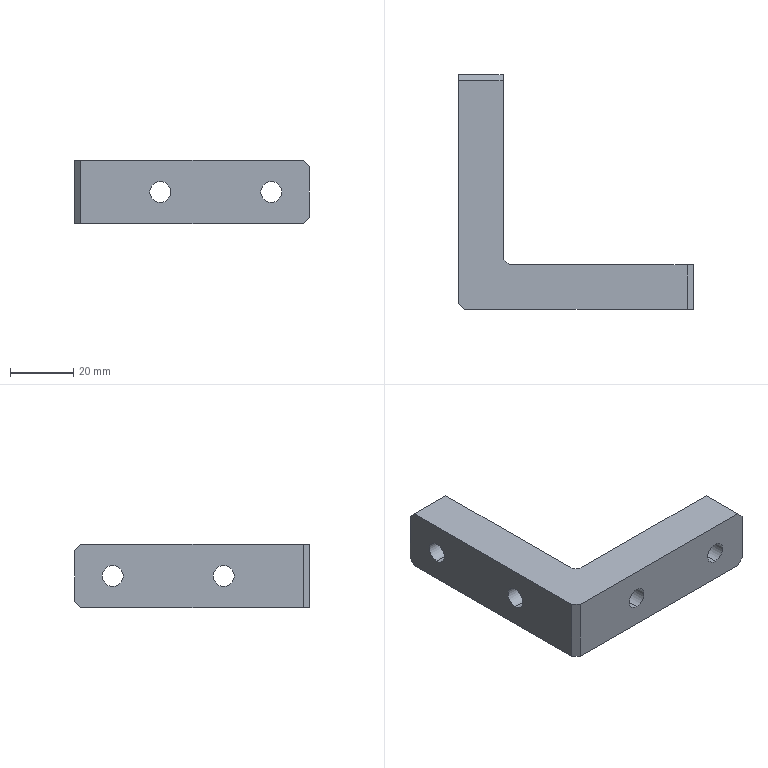Part | SolidWorks | features 3DProfileFeature 2, Chamfer 2, HoleWzd 2, Extrusion 1, Fillet 1 | 1 solid | 42 faces | box 74 x 74 x 20 mm | volume 33836 mm3 | cylinder 17 | plane 17 | cone 8 | commonest cylinder face diameters 6.6 x8 11 x8 6 x1
STEP:
#1=CARTESIAN_POINT('',(-12.,13.975,-5.5));
#2=VERTEX_POINT('',#1);
#3=CARTESIAN_POINT('',(-12.,13.975,5.5));
#4=VERTEX_POINT('',#3);
#5=CARTESIAN_POINT('',(-12.,13.975,0.));
#6=DIRECTION('',(0.,1.,0.));
#7=DIRECTION('',(0.,0.,1.));
#8=AXIS2_PLACEMENT_3D('',#5,#6,#7);
#9=CIRCLE('',#8,5.5);
#10=EDGE_CURVE('',#2,#4,#9,.T.);
#11=ORIENTED_EDGE('',*,*,#10,.F.);
#12=CARTESIAN_POINT('',(-12.,14.,-5.525));
#13=VERTEX_POINT('',#12);
#14=CARTESIAN_POINT('',(-12.,14.,-5.525));
#15=DIRECTION('',(0.,0.7071,-0.7071));
#16=VECTOR('',#15,1000.);
#17=LINE('',#14,#16);
#18=EDGE_CURVE('',#2,#13,#17,.T.);
#19=ORIENTED_EDGE('',*,*,#18,.T.);
#20=CARTESIAN_POINT('',(-12.,14.,5.525));
#21=VERTEX_POINT('',#20);
#22=CARTESIAN_POINT('',(-12.,14.,0.));
#23=DIRECTION('',(0.,1.,0.));
#24=DIRECTION('',(0.,0.,1.));
#25=AXIS2_PLACEMENT_3D('',#22,#23,#24);
#26=CIRCLE('',#25,5.525);
#27=EDGE_CURVE('',#13,#21,#26,.T.);
#28=ORIENTED_EDGE('',*,*,#27,.T.);
#29=CARTESIAN_POINT('',(-12.,14.,5.525));
#30=DIRECTION('',(0.,0.7071,0.7071));
#31=VECTOR('',#30,1000.);
#32=LINE('',#29,#31);
#33=EDGE_CURVE('',#4,#21,#32,.T.);
#34=ORIENTED_EDGE('',*,*,#33,.F.);
#35=EDGE_LOOP('',(#11,#19,#28,#34));
#36=FACE_OUTER_BOUND('',#35,.T.);
#37=CARTESIAN_POINT('',(-12.,14.,0.));
#38=DIRECTION('',(0.,1.,0.));
#39=DIRECTION('',(0.,0.,1.));
#40=AXIS2_PLACEMENT_3D('',#37,#38,#39);
#41=CONICAL_SURFACE('',#40,5.525,0.7854);
#42=ADVANCED_FACE('',(#36),#41,.F.);
#43=CARTESIAN_POINT('',(-12.,7.2,-5.5));
#44=VERTEX_POINT('',#43);
#45=CARTESIAN_POINT('',(-12.,7.2,5.5));
#46=VERTEX_POINT('',#45);
#47=CARTESIAN_POINT('',(-12.,7.2,0.));
#48=DIRECTION('',(0.,1.,0.));
#49=DIRECTION('',(0.,0.,1.));
#50=AXIS2_PLACEMENT_3D('',#47,#48,#49);
#51=CIRCLE('',#50,5.5);
#52=EDGE_CURVE('',#44,#46,#51,.T.);
#53=ORIENTED_EDGE('',*,*,#52,.F.);
#54=CARTESIAN_POINT('',(-12.,14.,-5.5));
#55=DIRECTION('',(0.,1.,0.));
#56=VECTOR('',#55,1000.);
#57=LINE('',#54,#56);
#58=EDGE_CURVE('',#44,#2,#57,.T.);
#59=ORIENTED_EDGE('',*,*,#58,.T.);
#60=ORIENTED_EDGE('',*,*,#10,.T.);
#61=CARTESIAN_POINT('',(-12.,14.,5.5));
#62=DIRECTION('',(0.,1.,0.));
#63=VECTOR('',#62,1000.);
#64=LINE('',#61,#63);
#65=EDGE_CURVE('',#46,#4,#64,.T.);
#66=ORIENTED_EDGE('',*,*,#65,.F.);
#67=EDGE_LOOP('',(#53,#59,#60,#66));
#68=FACE_OUTER_BOUND('',#67,.T.);
#69=CARTESIAN_POINT('',(-12.,14.,0.));
#70=DIRECTION('',(0.,1.,0.));
#71=DIRECTION('',(0.,0.,1.));
#72=AXIS2_PLACEMENT_3D('',#69,#70,#71);
#73=CYLINDRICAL_SURFACE('',#72,5.5);
#74=ADVANCED_FACE('',(#68),#73,.F.);
#75=CARTESIAN_POINT('',(-12.,0.,-3.3));
#76=VERTEX_POINT('',#75);
#77=CARTESIAN_POINT('',(-12.,0.,3.3));
#78=VERTEX_POINT('',#77);
#79=CARTESIAN_POINT('',(-12.,0.,0.));
#80=DIRECTION('',(0.,1.,0.));
#81=DIRECTION('',(-1.,0.,0.));
#82=AXIS2_PLACEMENT_3D('',#79,#80,#81);
#83=CIRCLE('',#82,3.3);
#84=EDGE_CURVE('',#76,#78,#83,.T.);
#85=ORIENTED_EDGE('',*,*,#84,.F.);
#86=CARTESIAN_POINT('',(-12.,7.2,-3.3));
#87=VERTEX_POINT('',#86);
#88=CARTESIAN_POINT('',(-12.,14.,-3.3));
#89=DIRECTION('',(0.,1.,0.));
#90=VECTOR('',#89,1000.);
#91=LINE('',#88,#90);
#92=EDGE_CURVE('',#76,#87,#91,.T.);
#93=ORIENTED_EDGE('',*,*,#92,.T.);
#94=CARTESIAN_POINT('',(-12.,7.2,3.3));
#95=VERTEX_POINT('',#94);
#96=CARTESIAN_POINT('',(-12.,7.2,0.));
#97=DIRECTION('',(0.,1.,0.));
#98=DIRECTION('',(0.,0.,1.));
#99=AXIS2_PLACEMENT_3D('',#96,#97,#98);
#100=CIRCLE('',#99,3.3);
#101=EDGE_CURVE('',#87,#95,#100,.T.);
#102=ORIENTED_EDGE('',*,*,#101,.T.);
#103=CARTESIAN_POINT('',(-12.,14.,3.3));
#104=DIRECTION('',(0.,1.,0.));
#105=VECTOR('',#104,1000.);
#106=LINE('',#103,#105);
#107=EDGE_CURVE('',#78,#95,#106,.T.);
#108=ORIENTED_EDGE('',*,*,#107,.F.);
#109=EDGE_LOOP('',(#85,#93,#102,#108));
#110=FACE_OUTER_BOUND('',#109,.T.);
#111=CARTESIAN_POINT('',(-12.,14.,0.));
#112=DIRECTION('',(0.,1.,0.));
#113=DIRECTION('',(0.,0.,1.));
#114=AXIS2_PLACEMENT_3D('',#111,#112,#113);
#115=CYLINDRICAL_SURFACE('',#114,3.3);
#116=ADVANCED_FACE('',(#110),#115,.F.);
#117=CARTESIAN_POINT('',(-47.,13.975,-5.5));
#118=VERTEX_POINT('',#117);
#119=CARTESIAN_POINT('',(-47.,13.975,5.5));
#120=VERTEX_POINT('',#119);
#121=CARTESIAN_POINT('',(-47.,13.975,0.));
#122=DIRECTION('',(0.,1.,0.));
#123=DIRECTION('',(0.,0.,1.));
#124=AXIS2_PLACEMENT_3D('',#121,#122,#123);
#125=CIRCLE('',#124,5.5);
#126=EDGE_CURVE('',#118,#120,#125,.T.);
#127=ORIENTED_EDGE('',*,*,#126,.F.);
#128=CARTESIAN_POINT('',(-47.,14.,-5.525));
#129=VERTEX_POINT('',#128);
#130=CARTESIAN_POINT('',(-47.,14.,-5.525));
#131=DIRECTION('',(0.,0.7071,-0.7071));
#132=VECTOR('',#131,1000.);
#133=LINE('',#130,#132);
#134=EDGE_CURVE('',#118,#129,#133,.T.);
#135=ORIENTED_EDGE('',*,*,#134,.T.);
#136=CARTESIAN_POINT('',(-47.,14.,5.525));
#137=VERTEX_POINT('',#136);
#138=CARTESIAN_POINT('',(-47.,14.,0.));
#139=DIRECTION('',(0.,1.,0.));
#140=DIRECTION('',(0.,0.,1.));
#141=AXIS2_PLACEMENT_3D('',#138,#139,#140);
#142=CIRCLE('',#141,5.525);
#143=EDGE_CURVE('',#129,#137,#142,.T.);
#144=ORIENTED_EDGE('',*,*,#143,.T.);
#145=CARTESIAN_POINT('',(-47.,14.,5.525));
#146=DIRECTION('',(0.,0.7071,0.7071));
#147=VECTOR('',#146,1000.);
#148=LINE('',#145,#147);
#149=EDGE_CURVE('',#120,#137,#148,.T.);
#150=ORIENTED_EDGE('',*,*,#149,.F.);
#151=EDGE_LOOP('',(#127,#135,#144,#150));
#152=FACE_OUTER_BOUND('',#151,.T.);
#153=CARTESIAN_POINT('',(-47.,14.,0.));
#154=DIRECTION('',(0.,1.,0.));
#155=DIRECTION('',(0.,0.,1.));
#156=AXIS2_PLACEMENT_3D('',#153,#154,#155);
#157=CONICAL_SURFACE('',#156,5.525,0.7854);
#158=ADVANCED_FACE('',(#152),#157,.F.);
#159=CARTESIAN_POINT('',(-47.,7.2,-5.5));
#160=VERTEX_POINT('',#159);
#161=CARTESIAN_POINT('',(-47.,7.2,5.5));
#162=VERTEX_POINT('',#161);
#163=CARTESIAN_POINT('',(-47.,7.2,0.));
#164=DIRECTION('',(0.,1.,0.));
#165=DIRECTION('',(0.,0.,1.));
#166=AXIS2_PLACEMENT_3D('',#163,#164,#165);
#167=CIRCLE('',#166,5.5);
#168=EDGE_CURVE('',#160,#162,#167,.T.);
#169=ORIENTED_EDGE('',*,*,#168,.F.);
#170=CARTESIAN_POINT('',(-47.,14.,-5.5));
#171=DIRECTION('',(0.,1.,0.));
#172=VECTOR('',#171,1000.);
#173=LINE('',#170,#172);
#174=EDGE_CURVE('',#160,#118,#173,.T.);
#175=ORIENTED_EDGE('',*,*,#174,.T.);
#176=ORIENTED_EDGE('',*,*,#126,.T.);
#177=CARTESIAN_POINT('',(-47.,14.,5.5));
#178=DIRECTION('',(0.,1.,0.));
#179=VECTOR('',#178,1000.);
#180=LINE('',#177,#179);
#181=EDGE_CURVE('',#162,#120,#180,.T.);
#182=ORIENTED_EDGE('',*,*,#181,.F.);
#183=EDGE_LOOP('',(#169,#175,#176,#182));
#184=FACE_OUTER_BOUND('',#183,.T.);
#185=CARTESIAN_POINT('',(-47.,14.,0.));
#186=DIRECTION('',(0.,1.,0.));
#187=DIRECTION('',(0.,0.,1.));
#188=AXIS2_PLACEMENT_3D('',#185,#186,#187);
#189=CYLINDRICAL_SURFACE('',#188,5.5);
#190=ADVANCED_FACE('',(#184),#189,.F.);
#191=CARTESIAN_POINT('',(-47.,0.,-3.3));
#192=VERTEX_POINT('',#191);
#193=CARTESIAN_POINT('',(-47.,0.,3.3));
#194=VERTEX_POINT('',#193);
#195=CARTESIAN_POINT('',(-47.,0.,0.));
#196=DIRECTION('',(0.,1.,0.));
#197=DIRECTION('',(-1.,0.,0.));
#198=AXIS2_PLACEMENT_3D('',#195,#196,#197);
#199=CIRCLE('',#198,3.3);
#200=EDGE_CURVE('',#192,#194,#199,.T.);
#201=ORIENTED_EDGE('',*,*,#200,.F.);
#202=CARTESIAN_POINT('',(-47.,7.2,-3.3));
#203=VERTEX_POINT('',#202);
#204=CARTESIAN_POINT('',(-47.,14.,-3.3));
#205=DIRECTION('',(0.,1.,0.));
#206=VECTOR('',#205,1000.);
#207=LINE('',#204,#206);
#208=EDGE_CURVE('',#192,#203,#207,.T.);
#209=ORIENTED_EDGE('',*,*,#208,.T.);
#210=CARTESIAN_POINT('',(-47.,7.2,3.3));
#211=VERTEX_POINT('',#210);
#212=CARTESIAN_POINT('',(-47.,7.2,0.));
#213=DIRECTION('',(0.,1.,0.));
#214=DIRECTION('',(0.,0.,1.));
#215=AXIS2_PLACEMENT_3D('',#212,#213,#214);
#216=CIRCLE('',#215,3.3);
#217=EDGE_CURVE('',#203,#211,#216,.T.);
#218=ORIENTED_EDGE('',*,*,#217,.T.);
#219=CARTESIAN_POINT('',(-47.,14.,3.3));
#220=DIRECTION('',(0.,1.,0.));
#221=VECTOR('',#220,1000.);
#222=LINE('',#219,#221);
#223=EDGE_CURVE('',#194,#211,#222,.T.);
#224=ORIENTED_EDGE('',*,*,#223,.F.);
#225=EDGE_LOOP('',(#201,#209,#218,#224));
#226=FACE_OUTER_BOUND('',#225,.T.);
#227=CARTESIAN_POINT('',(-47.,14.,0.));
#228=DIRECTION('',(0.,1.,0.));
#229=DIRECTION('',(0.,0.,1.));
#230=AXIS2_PLACEMENT_3D('',#227,#228,#229);
#231=CYLINDRICAL_SURFACE('',#230,3.3);
#232=ADVANCED_FACE('',(#226),#231,.F.);
#233=CARTESIAN_POINT('',(-60.025,62.,5.5));
#234=VERTEX_POINT('',#233);
#235=CARTESIAN_POINT('',(-60.025,62.,-5.5));
#236=VERTEX_POINT('',#235);
#237=CARTESIAN_POINT('',(-60.025,62.,0.));
#238=DIRECTION('',(1.,0.,0.));
#239=DIRECTION('',(0.,0.,-1.));
#240=AXIS2_PLACEMENT_3D('',#237,#238,#239);
#241=CIRCLE('',#240,5.5);
#242=EDGE_CURVE('',#234,#236,#241,.T.);
#243=ORIENTED_EDGE('',*,*,#242,.F.);
#244=CARTESIAN_POINT('',(-60.,62.,5.525));
#245=VERTEX_POINT('',#244);
#246=CARTESIAN_POINT('',(-60.,62.,5.525));
#247=DIRECTION('',(0.7071,0.,0.7071));
#248=VECTOR('',#247,1000.);
#249=LINE('',#246,#248);
#250=EDGE_CURVE('',#234,#245,#249,.T.);
#251=ORIENTED_EDGE('',*,*,#250,.T.);
#252=CARTESIAN_POINT('',(-60.,62.,-5.525));
#253=VERTEX_POINT('',#252);
#254=CARTESIAN_POINT('',(-60.,62.,0.));
#255=DIRECTION('',(1.,0.,0.));
#256=DIRECTION('',(0.,0.,-1.));
#257=AXIS2_PLACEMENT_3D('',#254,#255,#256);
#258=CIRCLE('',#257,5.525);
#259=EDGE_CURVE('',#245,#253,#258,.T.);
#260=ORIENTED_EDGE('',*,*,#259,.T.);
#261=CARTESIAN_POINT('',(-60.,62.,-5.525));
#262=DIRECTION('',(0.7071,0.,-0.7071));
#263=VECTOR('',#262,1000.);
#264=LINE('',#261,#263);
#265=EDGE_CURVE('',#236,#253,#264,.T.);
#266=ORIENTED_EDGE('',*,*,#265,.F.);
#267=EDGE_LOOP('',(#243,#251,#260,#266));
#268=FACE_OUTER_BOUND('',#267,.T.);
#269=CARTESIAN_POINT('',(-60.,62.,0.));
#270=DIRECTION('',(1.,0.,0.));
#271=DIRECTION('',(0.,0.,-1.));
#272=AXIS2_PLACEMENT_3D('',#269,#270,#271);
#273=CONICAL_SURFACE('',#272,5.525,0.7854);
#274=ADVANCED_FACE('',(#268),#273,.F.);
#275=CARTESIAN_POINT('',(-66.8,62.,5.5));
#276=VERTEX_POINT('',#275);
#277=CARTESIAN_POINT('',(-66.8,62.,-5.5));
#278=VERTEX_POINT('',#277);
#279=CARTESIAN_POINT('',(-66.8,62.,0.));
#280=DIRECTION('',(1.,0.,0.));
#281=DIRECTION('',(0.,0.,-1.));
#282=AXIS2_PLACEMENT_3D('',#279,#280,#281);
#283=CIRCLE('',#282,5.5);
#284=EDGE_CURVE('',#276,#278,#283,.T.);
#285=ORIENTED_EDGE('',*,*,#284,.F.);
#286=CARTESIAN_POINT('',(-60.,62.,5.5));
#287=DIRECTION('',(1.,0.,0.));
#288=VECTOR('',#287,1000.);
#289=LINE('',#286,#288);
#290=EDGE_CURVE('',#276,#234,#289,.T.);
#291=ORIENTED_EDGE('',*,*,#290,.T.);
#292=ORIENTED_EDGE('',*,*,#242,.T.);
#293=CARTESIAN_POINT('',(-60.,62.,-5.5));
#294=DIRECTION('',(1.,0.,0.));
#295=VECTOR('',#294,1000.);
#296=LINE('',#293,#295);
#297=EDGE_CURVE('',#278,#236,#296,.T.);
#298=ORIENTED_EDGE('',*,*,#297,.F.);
#299=EDGE_LOOP('',(#285,#291,#292,#298));
#300=FACE_OUTER_BOUND('',#299,.T.);
#301=CARTESIAN_POINT('',(-60.,62.,0.));
#302=DIRECTION('',(1.,0.,0.));
#303=DIRECTION('',(0.,0.,-1.));
#304=AXIS2_PLACEMENT_3D('',#301,#302,#303);
#305=CYLINDRICAL_SURFACE('',#304,5.5);
#306=ADVANCED_FACE('',(#300),#305,.F.);
#307=CARTESIAN_POINT('',(-74.,62.,3.3));
#308=VERTEX_POINT('',#307);
#309=CARTESIAN_POINT('',(-74.,62.,-3.3));
#310=VERTEX_POINT('',#309);
#311=CARTESIAN_POINT('',(-74.,62.,0.));
#312=DIRECTION('',(1.,0.,0.));
#313=DIRECTION('',(0.,0.,-1.));
#314=AXIS2_PLACEMENT_3D('',#311,#312,#313);
#315=CIRCLE('',#314,3.3);
#316=EDGE_CURVE('',#308,#310,#315,.T.);
#317=ORIENTED_EDGE('',*,*,#316,.F.);
#318=CARTESIAN_POINT('',(-66.8,62.,3.3));
#319=VERTEX_POINT('',#318);
#320=CARTESIAN_POINT('',(-60.,62.,3.3));
#321=DIRECTION('',(1.,0.,0.));
#322=VECTOR('',#321,1000.);
#323=LINE('',#320,#322);
#324=EDGE_CURVE('',#308,#319,#323,.T.);
#325=ORIENTED_EDGE('',*,*,#324,.T.);
#326=CARTESIAN_POINT('',(-66.8,62.,-3.3));
#327=VERTEX_POINT('',#326);
#328=CARTESIAN_POINT('',(-66.8,62.,0.));
#329=DIRECTION('',(1.,0.,0.));
#330=DIRECTION('',(0.,0.,-1.));
#331=AXIS2_PLACEMENT_3D('',#328,#329,#330);
#332=CIRCLE('',#331,3.3);
#333=EDGE_CURVE('',#319,#327,#332,.T.);
#334=ORIENTED_EDGE('',*,*,#333,.T.);
#335=CARTESIAN_POINT('',(-60.,62.,-3.3));
#336=DIRECTION('',(1.,0.,0.));
#337=VECTOR('',#336,1000.);
#338=LINE('',#335,#337);
#339=EDGE_CURVE('',#310,#327,#338,.T.);
#340=ORIENTED_EDGE('',*,*,#339,.F.);
#341=EDGE_LOOP('',(#317,#325,#334,#340));
#342=FACE_OUTER_BOUND('',#341,.T.);
#343=CARTESIAN_POINT('',(-60.,62.,0.));
#344=DIRECTION('',(1.,0.,0.));
#345=DIRECTION('',(0.,0.,-1.));
#346=AXIS2_PLACEMENT_3D('',#343,#344,#345);
#347=CYLINDRICAL_SURFACE('',#346,3.3);
#348=ADVANCED_FACE('',(#342),#347,.F.);
#349=CARTESIAN_POINT('',(-60.025,27.,5.5));
#350=VERTEX_POINT('',#349);
#351=CARTESIAN_POINT('',(-60.025,27.,-5.5));
#352=VERTEX_POINT('',#351);
#353=CARTESIAN_POINT('',(-60.025,27.,0.));
#354=DIRECTION('',(1.,0.,0.));
#355=DIRECTION('',(0.,0.,-1.));
#356=AXIS2_PLACEMENT_3D('',#353,#354,#355);
#357=CIRCLE('',#356,5.5);
#358=EDGE_CURVE('',#350,#352,#357,.T.);
#359=ORIENTED_EDGE('',*,*,#358,.F.);
#360=CARTESIAN_POINT('',(-60.,27.,5.525));
#361=VERTEX_POINT('',#360);
#362=CARTESIAN_POINT('',(-60.,27.,5.525));
#363=DIRECTION('',(0.7071,0.,0.7071));
#364=VECTOR('',#363,1000.);
#365=LINE('',#362,#364);
#366=EDGE_CURVE('',#350,#361,#365,.T.);
#367=ORIENTED_EDGE('',*,*,#366,.T.);
#368=CARTESIAN_POINT('',(-60.,27.,-5.525));
#369=VERTEX_POINT('',#368);
#370=CARTESIAN_POINT('',(-60.,27.,0.));
#371=DIRECTION('',(1.,0.,0.));
#372=DIRECTION('',(0.,0.,-1.));
#373=AXIS2_PLACEMENT_3D('',#370,#371,#372);
#374=CIRCLE('',#373,5.525);
#375=EDGE_CURVE('',#361,#369,#374,.T.);
#376=ORIENTED_EDGE('',*,*,#375,.T.);
#377=CARTESIAN_POINT('',(-60.,27.,-5.525));
#378=DIRECTION('',(0.7071,0.,-0.7071));
#379=VECTOR('',#378,1000.);
#380=LINE('',#377,#379);
#381=EDGE_CURVE('',#352,#369,#380,.T.);
#382=ORIENTED_EDGE('',*,*,#381,.F.);
#383=EDGE_LOOP('',(#359,#367,#376,#382));
#384=FACE_OUTER_BOUND('',#383,.T.);
#385=CARTESIAN_POINT('',(-60.,27.,0.));
#386=DIRECTION('',(1.,0.,0.));
#387=DIRECTION('',(0.,0.,-1.));
#388=AXIS2_PLACEMENT_3D('',#385,#386,#387);
#389=CONICAL_SURFACE('',#388,5.525,0.7854);
#390=ADVANCED_FACE('',(#384),#389,.F.);
#391=CARTESIAN_POINT('',(-66.8,27.,5.5));
#392=VERTEX_POINT('',#391);
#393=CARTESIAN_POINT('',(-66.8,27.,-5.5));
#394=VERTEX_POINT('',#393);
#395=CARTESIAN_POINT('',(-66.8,27.,0.));
#396=DIRECTION('',(1.,0.,0.));
#397=DIRECTION('',(0.,0.,-1.));
#398=AXIS2_PLACEMENT_3D('',#395,#396,#397);
#399=CIRCLE('',#398,5.5);
#400=EDGE_CURVE('',#392,#394,#399,.T.);
#401=ORIENTED_EDGE('',*,*,#400,.F.);
#402=CARTESIAN_POINT('',(-60.,27.,5.5));
#403=DIRECTION('',(1.,0.,0.));
#404=VECTOR('',#403,1000.);
#405=LINE('',#402,#404);
#406=EDGE_CURVE('',#392,#350,#405,.T.);
#407=ORIENTED_EDGE('',*,*,#406,.T.);
#408=ORIENTED_EDGE('',*,*,#358,.T.);
#409=CARTESIAN_POINT('',(-60.,27.,-5.5));
#410=DIRECTION('',(1.,0.,0.));
#411=VECTOR('',#410,1000.);
#412=LINE('',#409,#411);
#413=EDGE_CURVE('',#394,#352,#412,.T.);
#414=ORIENTED_EDGE('',*,*,#413,.F.);
#415=EDGE_LOOP('',(#401,#407,#408,#414));
#416=FACE_OUTER_BOUND('',#415,.T.);
#417=CARTESIAN_POINT('',(-60.,27.,0.));
#418=DIRECTION('',(1.,0.,0.));
#419=DIRECTION('',(0.,0.,-1.));
#420=AXIS2_PLACEMENT_3D('',#417,#418,#419);
#421=CYLINDRICAL_SURFACE('',#420,5.5);
#422=ADVANCED_FACE('',(#416),#421,.F.);
#423=CARTESIAN_POINT('',(-74.,27.,3.3));
#424=VERTEX_POINT('',#423);
#425=CARTESIAN_POINT('',(-74.,27.,-3.3));
#426=VERTEX_POINT('',#425);
#427=CARTESIAN_POINT('',(-74.,27.,0.));
#428=DIRECTION('',(1.,0.,0.));
#429=DIRECTION('',(0.,0.,-1.));
#430=AXIS2_PLACEMENT_3D('',#427,#428,#429);
#431=CIRCLE('',#430,3.3);
#432=EDGE_CURVE('',#424,#426,#431,.T.);
#433=ORIENTED_EDGE('',*,*,#432,.F.);
#434=CARTESIAN_POINT('',(-66.8,27.,3.3));
#435=VERTEX_POINT('',#434);
#436=CARTESIAN_POINT('',(-60.,27.,3.3));
#437=DIRECTION('',(1.,0.,0.));
#438=VECTOR('',#437,1000.);
#439=LINE('',#436,#438);
#440=EDGE_CURVE('',#424,#435,#439,.T.);
#441=ORIENTED_EDGE('',*,*,#440,.T.);
#442=CARTESIAN_POINT('',(-66.8,27.,-3.3));
#443=VERTEX_POINT('',#442);
#444=CARTESIAN_POINT('',(-66.8,27.,0.));
#445=DIRECTION('',(1.,0.,0.));
#446=DIRECTION('',(0.,0.,-1.));
#447=AXIS2_PLACEMENT_3D('',#444,#445,#446);
#448=CIRCLE('',#447,3.3);
#449=EDGE_CURVE('',#435,#443,#448,.T.);
#450=ORIENTED_EDGE('',*,*,#449,.T.);
#451=CARTESIAN_POINT('',(-60.,27.,-3.3));
#452=DIRECTION('',(1.,0.,0.));
#453=VECTOR('',#452,1000.);
#454=LINE('',#451,#453);
#455=EDGE_CURVE('',#426,#443,#454,.T.);
#456=ORIENTED_EDGE('',*,*,#455,.F.);
#457=EDGE_LOOP('',(#433,#441,#450,#456));
#458=FACE_OUTER_BOUND('',#457,.T.);
#459=CARTESIAN_POINT('',(-60.,27.,0.));
#460=DIRECTION('',(1.,0.,0.));
#461=DIRECTION('',(0.,0.,-1.));
#462=AXIS2_PLACEMENT_3D('',#459,#460,#461);
#463=CYLINDRICAL_SURFACE('',#462,3.3);
#464=ADVANCED_FACE('',(#458),#463,.F.);
#465=CARTESIAN_POINT('',(0.,14.,8.));
#466=VERTEX_POINT('',#465);
#467=CARTESIAN_POINT('',(0.,14.,-8.));
#468=VERTEX_POINT('',#467);
#469=CARTESIAN_POINT('',(0.,14.,10.));
#470=DIRECTION('',(0.,0.,-1.));
#471=VECTOR('',#470,1000.);
#472=LINE('',#469,#471);
#473=EDGE_CURVE('',#466,#468,#472,.T.);
#474=ORIENTED_EDGE('',*,*,#473,.F.);
#475=CARTESIAN_POINT('',(0.,0.,8.));
#476=VERTEX_POINT('',#475);
#477=CARTESIAN_POINT('',(0.,14.,8.));
#478=DIRECTION('',(0.,-1.,0.));
#479=VECTOR('',#478,1000.);
#480=LINE('',#477,#479);
#481=EDGE_CURVE('',#466,#476,#480,.T.);
#482=ORIENTED_EDGE('',*,*,#481,.T.);
#483=CARTESIAN_POINT('',(0.,0.,-8.));
#484=VERTEX_POINT('',#483);
#485=CARTESIAN_POINT('',(0.,0.,10.));
#486=DIRECTION('',(0.,0.,-1.));
#487=VECTOR('',#486,1000.);
#488=LINE('',#485,#487);
#489=EDGE_CURVE('',#476,#484,#488,.T.);
#490=ORIENTED_EDGE('',*,*,#489,.T.);
#491=CARTESIAN_POINT('',(0.,14.,-8.));
#492=DIRECTION('',(0.,1.,0.));
#493=VECTOR('',#492,1000.);
#494=LINE('',#491,#493);
#495=EDGE_CURVE('',#484,#468,#494,.T.);
#496=ORIENTED_EDGE('',*,*,#495,.T.);
#497=EDGE_LOOP('',(#474,#482,#490,#496));
#498=FACE_OUTER_BOUND('',#497,.T.);
#499=CARTESIAN_POINT('',(0.,14.,10.));
#500=DIRECTION('',(-1.,0.,0.));
#501=DIRECTION('',(0.,0.,1.));
#502=AXIS2_PLACEMENT_3D('',#499,#500,#501);
#503=PLANE('',#502);
#504=ADVANCED_FACE('',(#498),#503,.F.);
#505=CARTESIAN_POINT('',(-12.,14.,0.));
#506=DIRECTION('',(0.,1.,0.));
#507=DIRECTION('',(0.,0.,1.));
#508=AXIS2_PLACEMENT_3D('',#505,#506,#507);
#509=CIRCLE('',#508,5.525);
#510=EDGE_CURVE('',#21,#13,#509,.T.);
#511=ORIENTED_EDGE('',*,*,#510,.F.);
#512=ORIENTED_EDGE('',*,*,#27,.F.);
#513=EDGE_LOOP('',(#511,#512));
#514=FACE_BOUND('',#513,.T.);
#515=CARTESIAN_POINT('',(-47.,14.,0.));
#516=DIRECTION('',(0.,1.,0.));
#517=DIRECTION('',(0.,0.,1.));
#518=AXIS2_PLACEMENT_3D('',#515,#516,#517);
#519=CIRCLE('',#518,5.525);
#520=EDGE_CURVE('',#137,#129,#519,.T.);
#521=ORIENTED_EDGE('',*,*,#520,.F.);
#522=ORIENTED_EDGE('',*,*,#143,.F.);
#523=EDGE_LOOP('',(#521,#522));
#524=FACE_BOUND('',#523,.T.);
#525=CARTESIAN_POINT('',(-2.,14.,10.));
#526=VERTEX_POINT('',#525);
#527=CARTESIAN_POINT('',(-57.,14.,10.));
#528=VERTEX_POINT('',#527);
#529=CARTESIAN_POINT('',(-60.,14.,10.));
#530=DIRECTION('',(-1.,0.,0.));
#531=VECTOR('',#530,1000.);
#532=LINE('',#529,#531);
#533=EDGE_CURVE('',#526,#528,#532,.T.);
#534=ORIENTED_EDGE('',*,*,#533,.F.);
#535=CARTESIAN_POINT('',(-2.,14.,10.));
#536=DIRECTION('',(0.7071,0.,-0.7071));
#537=VECTOR('',#536,1000.);
#538=LINE('',#535,#537);
#539=EDGE_CURVE('',#526,#466,#538,.T.);
#540=ORIENTED_EDGE('',*,*,#539,.T.);
#541=ORIENTED_EDGE('',*,*,#473,.T.);
#542=CARTESIAN_POINT('',(-2.,14.,-10.));
#543=VERTEX_POINT('',#542);
#544=CARTESIAN_POINT('',(0.,14.,-8.));
#545=DIRECTION('',(-0.7071,0.,-0.7071));
#546=VECTOR('',#545,1000.);
#547=LINE('',#544,#546);
#548=EDGE_CURVE('',#468,#543,#547,.T.);
#549=ORIENTED_EDGE('',*,*,#548,.T.);
#550=CARTESIAN_POINT('',(-57.,14.,-10.));
#551=VERTEX_POINT('',#550);
#552=CARTESIAN_POINT('',(-60.,14.,-10.));
#553=DIRECTION('',(-1.,0.,0.));
#554=VECTOR('',#553,1000.);
#555=LINE('',#552,#554);
#556=EDGE_CURVE('',#543,#551,#555,.T.);
#557=ORIENTED_EDGE('',*,*,#556,.T.);
#558=CARTESIAN_POINT('',(-57.,14.,10.));
#559=DIRECTION('',(0.,0.,1.));
#560=VECTOR('',#559,1000.);
#561=LINE('',#558,#560);
#562=EDGE_CURVE('',#551,#528,#561,.T.);
#563=ORIENTED_EDGE('',*,*,#562,.T.);
#564=EDGE_LOOP('',(#534,#540,#541,#549,#557,#563));
#565=FACE_OUTER_BOUND('',#564,.T.);
#566=CARTESIAN_POINT('',(-60.,14.,10.));
#567=DIRECTION('',(0.,-1.,0.));
#568=DIRECTION('',(0.,0.,-1.));
#569=AXIS2_PLACEMENT_3D('',#566,#567,#568);
#570=PLANE('',#569);
#571=ADVANCED_FACE('',(#514,#524,#565),#570,.F.);
#572=CARTESIAN_POINT('',(-60.,62.,0.));
#573=DIRECTION('',(1.,0.,0.));
#574=DIRECTION('',(0.,0.,-1.));
#575=AXIS2_PLACEMENT_3D('',#572,#573,#574);
#576=CIRCLE('',#575,5.525);
#577=EDGE_CURVE('',#253,#245,#576,.T.);
#578=ORIENTED_EDGE('',*,*,#577,.F.);
#579=ORIENTED_EDGE('',*,*,#259,.F.);
#580=EDGE_LOOP('',(#578,#579));
#581=FACE_BOUND('',#580,.T.);
#582=CARTESIAN_POINT('',(-60.,27.,0.));
#583=DIRECTION('',(1.,0.,0.));
#584=DIRECTION('',(0.,0.,-1.));
#585=AXIS2_PLACEMENT_3D('',#582,#583,#584);
#586=CIRCLE('',#585,5.525);
#587=EDGE_CURVE('',#369,#361,#586,.T.);
#588=ORIENTED_EDGE('',*,*,#587,.F.);
#589=ORIENTED_EDGE('',*,*,#375,.F.);
#590=EDGE_LOOP('',(#588,#589));
#591=FACE_BOUND('',#590,.T.);
#592=CARTESIAN_POINT('',(-60.,74.,8.));
#593=VERTEX_POINT('',#592);
#594=CARTESIAN_POINT('',(-60.,74.,-8.));
#595=VERTEX_POINT('',#594);
#596=CARTESIAN_POINT('',(-60.,74.,10.));
#597=DIRECTION('',(0.,0.,-1.));
#598=VECTOR('',#597,1000.);
#599=LINE('',#596,#598);
#600=EDGE_CURVE('',#593,#595,#599,.T.);
#601=ORIENTED_EDGE('',*,*,#600,.F.);
#602=CARTESIAN_POINT('',(-60.,72.,10.));
#603=VERTEX_POINT('',#602);
#604=CARTESIAN_POINT('',(-60.,72.,10.));
#605=DIRECTION('',(0.,-0.7071,0.7071));
#606=VECTOR('',#605,1000.);
#607=LINE('',#604,#606);
#608=EDGE_CURVE('',#593,#603,#607,.T.);
#609=ORIENTED_EDGE('',*,*,#608,.T.);
#610=CARTESIAN_POINT('',(-60.,17.,10.));
#611=VERTEX_POINT('',#610);
#612=CARTESIAN_POINT('',(-60.,74.,10.));
#613=DIRECTION('',(0.,1.,0.));
#614=VECTOR('',#613,1000.);
#615=LINE('',#612,#614);
#616=EDGE_CURVE('',#611,#603,#615,.T.);
#617=ORIENTED_EDGE('',*,*,#616,.F.);
#618=CARTESIAN_POINT('',(-60.,17.,-10.));
#619=VERTEX_POINT('',#618);
#620=CARTESIAN_POINT('',(-60.,17.,-10.));
#621=DIRECTION('',(0.,0.,-1.));
#622=VECTOR('',#621,1000.);
#623=LINE('',#620,#622);
#624=EDGE_CURVE('',#611,#619,#623,.T.);
#625=ORIENTED_EDGE('',*,*,#624,.T.);
#626=CARTESIAN_POINT('',(-60.,72.,-10.));
#627=VERTEX_POINT('',#626);
#628=CARTESIAN_POINT('',(-60.,74.,-10.));
#629=DIRECTION('',(0.,1.,0.));
#630=VECTOR('',#629,1000.);
#631=LINE('',#628,#630);
#632=EDGE_CURVE('',#619,#627,#631,.T.);
#633=ORIENTED_EDGE('',*,*,#632,.T.);
#634=CARTESIAN_POINT('',(-60.,74.,-8.));
#635=DIRECTION('',(0.,0.7071,0.7071));
#636=VECTOR('',#635,1000.);
#637=LINE('',#634,#636);
#638=EDGE_CURVE('',#627,#595,#637,.T.);
#639=ORIENTED_EDGE('',*,*,#638,.T.);
#640=EDGE_LOOP('',(#601,#609,#617,#625,#633,#639));
#641=FACE_OUTER_BOUND('',#640,.T.);
#642=CARTESIAN_POINT('',(-60.,74.,10.));
#643=DIRECTION('',(-1.,0.,0.));
#644=DIRECTION('',(0.,-1.,0.));
#645=AXIS2_PLACEMENT_3D('',#642,#643,#644);
#646=PLANE('',#645);
#647=ADVANCED_FACE('',(#581,#591,#641),#646,.F.);
#648=CARTESIAN_POINT('',(-74.,74.,8.));
#649=VERTEX_POINT('',#648);
#650=CARTESIAN_POINT('',(-74.,74.,-8.));
#651=VERTEX_POINT('',#650);
#652=CARTESIAN_POINT('',(-74.,74.,10.));
#653=DIRECTION('',(0.,0.,-1.));
#654=VECTOR('',#653,1000.);
#655=LINE('',#652,#654);
#656=EDGE_CURVE('',#649,#651,#655,.T.);
#657=ORIENTED_EDGE('',*,*,#656,.F.);
#658=CARTESIAN_POINT('',(-74.,74.,8.));
#659=DIRECTION('',(1.,0.,0.));
#660=VECTOR('',#659,1000.);
#661=LINE('',#658,#660);
#662=EDGE_CURVE('',#649,#593,#661,.T.);
#663=ORIENTED_EDGE('',*,*,#662,.T.);
#664=ORIENTED_EDGE('',*,*,#600,.T.);
#665=CARTESIAN_POINT('',(-74.,74.,-8.));
#666=DIRECTION('',(-1.,0.,0.));
#667=VECTOR('',#666,1000.);
#668=LINE('',#665,#667);
#669=EDGE_CURVE('',#595,#651,#668,.T.);
#670=ORIENTED_EDGE('',*,*,#669,.T.);
#671=EDGE_LOOP('',(#657,#663,#664,#670));
#672=FACE_OUTER_BOUND('',#671,.T.);
#673=CARTESIAN_POINT('',(-74.,74.,10.));
#674=DIRECTION('',(0.,-1.,0.));
#675=DIRECTION('',(0.,0.,-1.));
#676=AXIS2_PLACEMENT_3D('',#673,#674,#675);
#677=PLANE('',#676);
#678=ADVANCED_FACE('',(#672),#677,.F.);
#679=CARTESIAN_POINT('',(-74.,62.,0.));
#680=DIRECTION('',(1.,0.,0.));
#681=DIRECTION('',(0.,0.,-1.));
#682=AXIS2_PLACEMENT_3D('',#679,#680,#681);
#683=CIRCLE('',#682,3.3);
#684=EDGE_CURVE('',#310,#308,#683,.T.);
#685=ORIENTED_EDGE('',*,*,#684,.T.);
#686=ORIENTED_EDGE('',*,*,#316,.T.);
#687=EDGE_LOOP('',(#685,#686));
#688=FACE_BOUND('',#687,.T.);
#689=CARTESIAN_POINT('',(-74.,27.,0.));
#690=DIRECTION('',(1.,0.,0.));
#691=DIRECTION('',(0.,0.,-1.));
#692=AXIS2_PLACEMENT_3D('',#689,#690,#691);
#693=CIRCLE('',#692,3.3);
#694=EDGE_CURVE('',#426,#424,#693,.T.);
#695=ORIENTED_EDGE('',*,*,#694,.T.);
#696=ORIENTED_EDGE('',*,*,#432,.T.);
#697=EDGE_LOOP('',(#695,#696));
#698=FACE_BOUND('',#697,.T.);
#699=CARTESIAN_POINT('',(-74.,72.,-10.));
#700=VERTEX_POINT('',#699);
#701=CARTESIAN_POINT('',(-74.,2.,-10.));
#702=VERTEX_POINT('',#701);
#703=CARTESIAN_POINT('',(-74.,0.,-10.));
#704=DIRECTION('',(0.,-1.,0.));
#705=VECTOR('',#704,1000.);
#706=LINE('',#703,#705);
#707=EDGE_CURVE('',#700,#702,#706,.T.);
#708=ORIENTED_EDGE('',*,*,#707,.T.);
#709=CARTESIAN_POINT('',(-74.,2.,10.));
#710=VERTEX_POINT('',#709);
#711=CARTESIAN_POINT('',(-74.,2.,10.));
#712=DIRECTION('',(0.,0.,1.));
#713=VECTOR('',#712,1000.);
#714=LINE('',#711,#713);
#715=EDGE_CURVE('',#702,#710,#714,.T.);
#716=ORIENTED_EDGE('',*,*,#715,.T.);
#717=CARTESIAN_POINT('',(-74.,72.,10.));
#718=VERTEX_POINT('',#717);
#719=CARTESIAN_POINT('',(-74.,0.,10.));
#720=DIRECTION('',(0.,-1.,0.));
#721=VECTOR('',#720,1000.);
#722=LINE('',#719,#721);
#723=EDGE_CURVE('',#718,#710,#722,.T.);
#724=ORIENTED_EDGE('',*,*,#723,.F.);
#725=CARTESIAN_POINT('',(-74.,72.,10.));
#726=DIRECTION('',(0.,0.7071,-0.7071));
#727=VECTOR('',#726,1000.);
#728=LINE('',#725,#727);
#729=EDGE_CURVE('',#718,#649,#728,.T.);
#730=ORIENTED_EDGE('',*,*,#729,.T.);
#731=ORIENTED_EDGE('',*,*,#656,.T.);
#732=CARTESIAN_POINT('',(-74.,74.,-8.));
#733=DIRECTION('',(0.,-0.7071,-0.7071));
#734=VECTOR('',#733,1000.);
#735=LINE('',#732,#734);
#736=EDGE_CURVE('',#651,#700,#735,.T.);
#737=ORIENTED_EDGE('',*,*,#736,.T.);
#738=EDGE_LOOP('',(#708,#716,#724,#730,#731,#737));
#739=FACE_OUTER_BOUND('',#738,.T.);
#740=CARTESIAN_POINT('',(-74.,0.,10.));
#741=DIRECTION('',(1.,0.,0.));
#742=DIRECTION('',(0.,0.,-1.));
#743=AXIS2_PLACEMENT_3D('',#740,#741,#742);
#744=PLANE('',#743);
#745=ADVANCED_FACE('',(#688,#698,#739),#744,.F.);
#746=CARTESIAN_POINT('',(-12.,0.,0.));
#747=DIRECTION('',(0.,1.,0.));
#748=DIRECTION('',(-1.,0.,0.));
#749=AXIS2_PLACEMENT_3D('',#746,#747,#748);
#750=CIRCLE('',#749,3.3);
#751=EDGE_CURVE('',#78,#76,#750,.T.);
#752=ORIENTED_EDGE('',*,*,#751,.T.);
#753=ORIENTED_EDGE('',*,*,#84,.T.);
#754=EDGE_LOOP('',(#752,#753));
#755=FACE_BOUND('',#754,.T.);
#756=CARTESIAN_POINT('',(-47.,0.,0.));
#757=DIRECTION('',(0.,1.,0.));
#758=DIRECTION('',(-1.,0.,0.));
#759=AXIS2_PLACEMENT_3D('',#756,#757,#758);
#760=CIRCLE('',#759,3.3);
#761=EDGE_CURVE('',#194,#192,#760,.T.);
#762=ORIENTED_EDGE('',*,*,#761,.T.);
#763=ORIENTED_EDGE('',*,*,#200,.T.);
#764=EDGE_LOOP('',(#762,#763));
#765=FACE_BOUND('',#764,.T.);
#766=CARTESIAN_POINT('',(-72.,0.,10.));
#767=VERTEX_POINT('',#766);
#768=CARTESIAN_POINT('',(-2.,0.,10.));
#769=VERTEX_POINT('',#768);
#770=CARTESIAN_POINT('',(0.,0.,10.));
#771=DIRECTION('',(1.,0.,0.));
#772=VECTOR('',#771,1000.);
#773=LINE('',#770,#772);
#774=EDGE_CURVE('',#767,#769,#773,.T.);
#775=ORIENTED_EDGE('',*,*,#774,.F.);
#776=CARTESIAN_POINT('',(-72.,0.,-10.));
#777=VERTEX_POINT('',#776);
#778=CARTESIAN_POINT('',(-72.,0.,10.));
#779=DIRECTION('',(0.,0.,-1.));
#780=VECTOR('',#779,1000.);
#781=LINE('',#778,#780);
#782=EDGE_CURVE('',#767,#777,#781,.T.);
#783=ORIENTED_EDGE('',*,*,#782,.T.);
#784=CARTESIAN_POINT('',(-2.,0.,-10.));
#785=VERTEX_POINT('',#784);
#786=CARTESIAN_POINT('',(0.,0.,-10.));
#787=DIRECTION('',(1.,0.,0.));
#788=VECTOR('',#787,1000.);
#789=LINE('',#786,#788);
#790=EDGE_CURVE('',#777,#785,#789,.T.);
#791=ORIENTED_EDGE('',*,*,#790,.T.);
#792=CARTESIAN_POINT('',(0.,0.,-8.));
#793=DIRECTION('',(0.7071,0.,0.7071));
#794=VECTOR('',#793,1000.);
#795=LINE('',#792,#794);
#796=EDGE_CURVE('',#785,#484,#795,.T.);
#797=ORIENTED_EDGE('',*,*,#796,.T.);
#798=ORIENTED_EDGE('',*,*,#489,.F.);
#799=CARTESIAN_POINT('',(-2.,0.,10.));
#800=DIRECTION('',(-0.7071,0.,0.7071));
#801=VECTOR('',#800,1000.);
#802=LINE('',#799,#801);
#803=EDGE_CURVE('',#476,#769,#802,.T.);
#804=ORIENTED_EDGE('',*,*,#803,.T.);
#805=EDGE_LOOP('',(#775,#783,#791,#797,#798,#804));
#806=FACE_OUTER_BOUND('',#805,.T.);
#807=CARTESIAN_POINT('',(0.,0.,10.));
#808=DIRECTION('',(0.,1.,0.));
#809=DIRECTION('',(-1.,0.,0.));
#810=AXIS2_PLACEMENT_3D('',#807,#808,#809);
#811=PLANE('',#810);
#812=ADVANCED_FACE('',(#755,#765,#806),#811,.F.);
#813=ORIENTED_EDGE('',*,*,#723,.T.);
#814=CARTESIAN_POINT('',(-72.,0.,10.));
#815=DIRECTION('',(0.7071,-0.7071,0.));
#816=VECTOR('',#815,1000.);
#817=LINE('',#814,#816);
#818=EDGE_CURVE('',#710,#767,#817,.T.);
#819=ORIENTED_EDGE('',*,*,#818,.T.);
#820=ORIENTED_EDGE('',*,*,#774,.T.);
#821=CARTESIAN_POINT('',(-2.,0.,10.));
#822=DIRECTION('',(0.,1.,0.));
#823=VECTOR('',#822,1000.);
#824=LINE('',#821,#823);
#825=EDGE_CURVE('',#769,#526,#824,.T.);
#826=ORIENTED_EDGE('',*,*,#825,.T.);
#827=ORIENTED_EDGE('',*,*,#533,.T.);
#828=CARTESIAN_POINT('',(-57.,17.,10.));
#829=DIRECTION('',(0.,0.,-1.));
#830=DIRECTION('',(-1.,0.,0.));
#831=AXIS2_PLACEMENT_3D('',#828,#829,#830);
#832=CIRCLE('',#831,3.);
#833=EDGE_CURVE('',#528,#611,#832,.T.);
#834=ORIENTED_EDGE('',*,*,#833,.T.);
#835=ORIENTED_EDGE('',*,*,#616,.T.);
#836=CARTESIAN_POINT('',(0.,72.,10.));
#837=DIRECTION('',(-1.,0.,0.));
#838=VECTOR('',#837,1000.);
#839=LINE('',#836,#838);
#840=EDGE_CURVE('',#603,#718,#839,.T.);
#841=ORIENTED_EDGE('',*,*,#840,.T.);
#842=EDGE_LOOP('',(#813,#819,#820,#826,#827,#834,#835,#841));
#843=FACE_OUTER_BOUND('',#842,.T.);
#844=CARTESIAN_POINT('',(0.,0.,10.));
#845=DIRECTION('',(0.,0.,-1.));
#846=DIRECTION('',(-1.,0.,0.));
#847=AXIS2_PLACEMENT_3D('',#844,#845,#846);
#848=PLANE('',#847);
#849=ADVANCED_FACE('',(#843),#848,.F.);
#850=ORIENTED_EDGE('',*,*,#790,.F.);
#851=CARTESIAN_POINT('',(-36.,-36.,-10.));
#852=DIRECTION('',(-0.7071,0.7071,0.));
#853=VECTOR('',#852,1000.);
#854=LINE('',#851,#853);
#855=EDGE_CURVE('',#777,#702,#854,.T.);
#856=ORIENTED_EDGE('',*,*,#855,.T.);
#857=ORIENTED_EDGE('',*,*,#707,.F.);
#858=CARTESIAN_POINT('',(-60.,72.,-10.));
#859=DIRECTION('',(1.,0.,0.));
#860=VECTOR('',#859,1000.);
#861=LINE('',#858,#860);
#862=EDGE_CURVE('',#700,#627,#861,.T.);
#863=ORIENTED_EDGE('',*,*,#862,.T.);
#864=ORIENTED_EDGE('',*,*,#632,.F.);
#865=CARTESIAN_POINT('',(-57.,17.,-10.));
#866=DIRECTION('',(0.,0.,1.));
#867=DIRECTION('',(-1.,0.,0.));
#868=AXIS2_PLACEMENT_3D('',#865,#866,#867);
#869=CIRCLE('',#868,3.);
#870=EDGE_CURVE('',#619,#551,#869,.T.);
#871=ORIENTED_EDGE('',*,*,#870,.T.);
#872=ORIENTED_EDGE('',*,*,#556,.F.);
#873=CARTESIAN_POINT('',(-2.,0.,-10.));
#874=DIRECTION('',(0.,-1.,0.));
#875=VECTOR('',#874,1000.);
#876=LINE('',#873,#875);
#877=EDGE_CURVE('',#543,#785,#876,.T.);
#878=ORIENTED_EDGE('',*,*,#877,.T.);
#879=EDGE_LOOP('',(#850,#856,#857,#863,#864,#871,#872,#878));
#880=FACE_OUTER_BOUND('',#879,.T.);
#881=CARTESIAN_POINT('',(0.,0.,-10.));
#882=DIRECTION('',(0.,0.,-1.));
#883=DIRECTION('',(-1.,0.,0.));
#884=AXIS2_PLACEMENT_3D('',#881,#882,#883);
#885=PLANE('',#884);
#886=ADVANCED_FACE('',(#880),#885,.T.);
#887=ORIENTED_EDGE('',*,*,#833,.F.);
#888=ORIENTED_EDGE('',*,*,#562,.F.);
#889=ORIENTED_EDGE('',*,*,#870,.F.);
#890=ORIENTED_EDGE('',*,*,#624,.F.);
#891=EDGE_LOOP('',(#887,#888,#889,#890));
#892=FACE_OUTER_BOUND('',#891,.T.);
#893=CARTESIAN_POINT('',(-57.,17.,10.));
#894=DIRECTION('',(0.,0.,1.));
#895=DIRECTION('',(1.,0.,0.));
#896=AXIS2_PLACEMENT_3D('',#893,#894,#895);
#897=CYLINDRICAL_SURFACE('',#896,3.);
#898=ADVANCED_FACE('',(#892),#897,.F.);
#899=ORIENTED_EDGE('',*,*,#803,.F.);
#900=ORIENTED_EDGE('',*,*,#481,.F.);
#901=ORIENTED_EDGE('',*,*,#539,.F.);
#902=ORIENTED_EDGE('',*,*,#825,.F.);
#903=EDGE_LOOP('',(#899,#900,#901,#902));
#904=FACE_OUTER_BOUND('',#903,.T.);
#905=CARTESIAN_POINT('',(-2.,0.,10.));
#906=DIRECTION('',(-0.7071,0.,-0.7071));
#907=DIRECTION('',(0.,1.,0.));
#908=AXIS2_PLACEMENT_3D('',#905,#906,#907);
#909=PLANE('',#908);
#910=ADVANCED_FACE('',(#904),#909,.F.);
#911=ORIENTED_EDGE('',*,*,#796,.F.);
#912=ORIENTED_EDGE('',*,*,#877,.F.);
#913=ORIENTED_EDGE('',*,*,#548,.F.);
#914=ORIENTED_EDGE('',*,*,#495,.F.);
#915=EDGE_LOOP('',(#911,#912,#913,#914));
#916=FACE_OUTER_BOUND('',#915,.T.);
#917=CARTESIAN_POINT('',(0.,14.,-8.));
#918=DIRECTION('',(0.7071,0.,-0.7071));
#919=DIRECTION('',(0.,-1.,0.));
#920=AXIS2_PLACEMENT_3D('',#917,#918,#919);
#921=PLANE('',#920);
#922=ADVANCED_FACE('',(#916),#921,.T.);
#923=ORIENTED_EDGE('',*,*,#608,.F.);
#924=ORIENTED_EDGE('',*,*,#662,.F.);
#925=ORIENTED_EDGE('',*,*,#729,.F.);
#926=ORIENTED_EDGE('',*,*,#840,.F.);
#927=EDGE_LOOP('',(#923,#924,#925,#926));
#928=FACE_OUTER_BOUND('',#927,.T.);
#929=CARTESIAN_POINT('',(0.,72.,10.));
#930=DIRECTION('',(0.,-0.7071,-0.7071));
#931=DIRECTION('',(-1.,0.,0.));
#932=AXIS2_PLACEMENT_3D('',#929,#930,#931);
#933=PLANE('',#932);
#934=ADVANCED_FACE('',(#928),#933,.F.);
#935=ORIENTED_EDGE('',*,*,#638,.F.);
#936=ORIENTED_EDGE('',*,*,#862,.F.);
#937=ORIENTED_EDGE('',*,*,#736,.F.);
#938=ORIENTED_EDGE('',*,*,#669,.F.);
#939=EDGE_LOOP('',(#935,#936,#937,#938));
#940=FACE_OUTER_BOUND('',#939,.T.);
#941=CARTESIAN_POINT('',(-74.,74.,-8.));
#942=DIRECTION('',(0.,0.7071,-0.7071));
#943=DIRECTION('',(1.,0.,0.));
#944=AXIS2_PLACEMENT_3D('',#941,#942,#943);
#945=PLANE('',#944);
#946=ADVANCED_FACE('',(#940),#945,.T.);
#947=ORIENTED_EDGE('',*,*,#818,.F.);
#948=ORIENTED_EDGE('',*,*,#715,.F.);
#949=ORIENTED_EDGE('',*,*,#855,.F.);
#950=ORIENTED_EDGE('',*,*,#782,.F.);
#951=EDGE_LOOP('',(#947,#948,#949,#950));
#952=FACE_OUTER_BOUND('',#951,.T.);
#953=CARTESIAN_POINT('',(-72.,0.,10.));
#954=DIRECTION('',(0.7071,0.7071,0.));
#955=DIRECTION('',(0.,0.,-1.));
#956=AXIS2_PLACEMENT_3D('',#953,#954,#955);
#957=PLANE('',#956);
#958=ADVANCED_FACE('',(#952),#957,.F.);
#959=ORIENTED_EDGE('',*,*,#440,.F.);
#960=ORIENTED_EDGE('',*,*,#694,.F.);
#961=ORIENTED_EDGE('',*,*,#455,.T.);
#962=CARTESIAN_POINT('',(-66.8,27.,0.));
#963=DIRECTION('',(1.,0.,0.));
#964=DIRECTION('',(0.,0.,-1.));
#965=AXIS2_PLACEMENT_3D('',#962,#963,#964);
#966=CIRCLE('',#965,3.3);
#967=EDGE_CURVE('',#443,#435,#966,.T.);
#968=ORIENTED_EDGE('',*,*,#967,.T.);
#969=EDGE_LOOP('',(#959,#960,#961,#968));
#970=FACE_OUTER_BOUND('',#969,.T.);
#971=CARTESIAN_POINT('',(-60.,27.,0.));
#972=DIRECTION('',(1.,0.,0.));
#973=DIRECTION('',(0.,0.,-1.));
#974=AXIS2_PLACEMENT_3D('',#971,#972,#973);
#975=CYLINDRICAL_SURFACE('',#974,3.3);
#976=ADVANCED_FACE('',(#970),#975,.F.);
#977=ORIENTED_EDGE('',*,*,#967,.F.);
#978=ORIENTED_EDGE('',*,*,#449,.F.);
#979=EDGE_LOOP('',(#977,#978));
#980=FACE_BOUND('',#979,.T.);
#981=CARTESIAN_POINT('',(-66.8,27.,0.));
#982=DIRECTION('',(1.,0.,0.));
#983=DIRECTION('',(0.,0.,-1.));
#984=AXIS2_PLACEMENT_3D('',#981,#982,#983);
#985=CIRCLE('',#984,5.5);
#986=EDGE_CURVE('',#394,#392,#985,.T.);
#987=ORIENTED_EDGE('',*,*,#986,.T.);
#988=ORIENTED_EDGE('',*,*,#400,.T.);
#989=EDGE_LOOP('',(#987,#988));
#990=FACE_OUTER_BOUND('',#989,.T.);
#991=CARTESIAN_POINT('',(-66.8,32.5,0.));
#992=DIRECTION('',(-1.,0.,0.));
#993=DIRECTION('',(0.,0.,1.));
#994=AXIS2_PLACEMENT_3D('',#991,#992,#993);
#995=PLANE('',#994);
#996=ADVANCED_FACE('',(#980,#990),#995,.F.);
#997=ORIENTED_EDGE('',*,*,#406,.F.);
#998=ORIENTED_EDGE('',*,*,#986,.F.);
#999=ORIENTED_EDGE('',*,*,#413,.T.);
#1000=CARTESIAN_POINT('',(-60.025,27.,0.));
#1001=DIRECTION('',(1.,0.,0.));
#1002=DIRECTION('',(0.,0.,-1.));
#1003=AXIS2_PLACEMENT_3D('',#1000,#1001,#1002);
#1004=CIRCLE('',#1003,5.5);
#1005=EDGE_CURVE('',#352,#350,#1004,.T.);
#1006=ORIENTED_EDGE('',*,*,#1005,.T.);
#1007=EDGE_LOOP('',(#997,#998,#999,#1006));
#1008=FACE_OUTER_BOUND('',#1007,.T.);
#1009=CARTESIAN_POINT('',(-60.,27.,0.));
#1010=DIRECTION('',(1.,0.,0.));
#1011=DIRECTION('',(0.,0.,-1.));
#1012=AXIS2_PLACEMENT_3D('',#1009,#1010,#1011);
#1013=CYLINDRICAL_SURFACE('',#1012,5.5);
#1014=ADVANCED_FACE('',(#1008),#1013,.F.);
#1015=ORIENTED_EDGE('',*,*,#366,.F.);
#1016=ORIENTED_EDGE('',*,*,#1005,.F.);
#1017=ORIENTED_EDGE('',*,*,#381,.T.);
#1018=ORIENTED_EDGE('',*,*,#587,.T.);
#1019=EDGE_LOOP('',(#1015,#1016,#1017,#1018));
#1020=FACE_OUTER_BOUND('',#1019,.T.);
#1021=CARTESIAN_POINT('',(-60.,27.,0.));
#1022=DIRECTION('',(1.,0.,0.));
#1023=DIRECTION('',(0.,0.,-1.));
#1024=AXIS2_PLACEMENT_3D('',#1021,#1022,#1023);
#1025=CONICAL_SURFACE('',#1024,5.525,0.7854);
#1026=ADVANCED_FACE('',(#1020),#1025,.F.);
#1027=ORIENTED_EDGE('',*,*,#324,.F.);
#1028=ORIENTED_EDGE('',*,*,#684,.F.);
#1029=ORIENTED_EDGE('',*,*,#339,.T.);
#1030=CARTESIAN_POINT('',(-66.8,62.,0.));
#1031=DIRECTION('',(1.,0.,0.));
#1032=DIRECTION('',(0.,0.,-1.));
#1033=AXIS2_PLACEMENT_3D('',#1030,#1031,#1032);
#1034=CIRCLE('',#1033,3.3);
#1035=EDGE_CURVE('',#327,#319,#1034,.T.);
#1036=ORIENTED_EDGE('',*,*,#1035,.T.);
#1037=EDGE_LOOP('',(#1027,#1028,#1029,#1036));
#1038=FACE_OUTER_BOUND('',#1037,.T.);
#1039=CARTESIAN_POINT('',(-60.,62.,0.));
#1040=DIRECTION('',(1.,0.,0.));
#1041=DIRECTION('',(0.,0.,-1.));
#1042=AXIS2_PLACEMENT_3D('',#1039,#1040,#1041);
#1043=CYLINDRICAL_SURFACE('',#1042,3.3);
#1044=ADVANCED_FACE('',(#1038),#1043,.F.);
#1045=ORIENTED_EDGE('',*,*,#1035,.F.);
#1046=ORIENTED_EDGE('',*,*,#333,.F.);
#1047=EDGE_LOOP('',(#1045,#1046));
#1048=FACE_BOUND('',#1047,.T.);
#1049=CARTESIAN_POINT('',(-66.8,62.,0.));
#1050=DIRECTION('',(1.,0.,0.));
#1051=DIRECTION('',(0.,0.,-1.));
#1052=AXIS2_PLACEMENT_3D('',#1049,#1050,#1051);
#1053=CIRCLE('',#1052,5.5);
#1054=EDGE_CURVE('',#278,#276,#1053,.T.);
#1055=ORIENTED_EDGE('',*,*,#1054,.T.);
#1056=ORIENTED_EDGE('',*,*,#284,.T.);
#1057=EDGE_LOOP('',(#1055,#1056));
#1058=FACE_OUTER_BOUND('',#1057,.T.);
#1059=CARTESIAN_POINT('',(-66.8,67.5,0.));
#1060=DIRECTION('',(-1.,0.,0.));
#1061=DIRECTION('',(0.,0.,1.));
#1062=AXIS2_PLACEMENT_3D('',#1059,#1060,#1061);
#1063=PLANE('',#1062);
#1064=ADVANCED_FACE('',(#1048,#1058),#1063,.F.);
#1065=ORIENTED_EDGE('',*,*,#290,.F.);
#1066=ORIENTED_EDGE('',*,*,#1054,.F.);
#1067=ORIENTED_EDGE('',*,*,#297,.T.);
#1068=CARTESIAN_POINT('',(-60.025,62.,0.));
#1069=DIRECTION('',(1.,0.,0.));
#1070=DIRECTION('',(0.,0.,-1.));
#1071=AXIS2_PLACEMENT_3D('',#1068,#1069,#1070);
#1072=CIRCLE('',#1071,5.5);
#1073=EDGE_CURVE('',#236,#234,#1072,.T.);
#1074=ORIENTED_EDGE('',*,*,#1073,.T.);
#1075=EDGE_LOOP('',(#1065,#1066,#1067,#1074));
#1076=FACE_OUTER_BOUND('',#1075,.T.);
#1077=CARTESIAN_POINT('',(-60.,62.,0.));
#1078=DIRECTION('',(1.,0.,0.));
#1079=DIRECTION('',(0.,0.,-1.));
#1080=AXIS2_PLACEMENT_3D('',#1077,#1078,#1079);
#1081=CYLINDRICAL_SURFACE('',#1080,5.5);
#1082=ADVANCED_FACE('',(#1076),#1081,.F.);
#1083=ORIENTED_EDGE('',*,*,#250,.F.);
#1084=ORIENTED_EDGE('',*,*,#1073,.F.);
#1085=ORIENTED_EDGE('',*,*,#265,.T.);
#1086=ORIENTED_EDGE('',*,*,#577,.T.);
#1087=EDGE_LOOP('',(#1083,#1084,#1085,#1086));
#1088=FACE_OUTER_BOUND('',#1087,.T.);
#1089=CARTESIAN_POINT('',(-60.,62.,0.));
#1090=DIRECTION('',(1.,0.,0.));
#1091=DIRECTION('',(0.,0.,-1.));
#1092=AXIS2_PLACEMENT_3D('',#1089,#1090,#1091);
#1093=CONICAL_SURFACE('',#1092,5.525,0.7854);
#1094=ADVANCED_FACE('',(#1088),#1093,.F.);
#1095=ORIENTED_EDGE('',*,*,#208,.F.);
#1096=ORIENTED_EDGE('',*,*,#761,.F.);
#1097=ORIENTED_EDGE('',*,*,#223,.T.);
#1098=CARTESIAN_POINT('',(-47.,7.2,0.));
#1099=DIRECTION('',(0.,1.,0.));
#1100=DIRECTION('',(0.,0.,1.));
#1101=AXIS2_PLACEMENT_3D('',#1098,#1099,#1100);
#1102=CIRCLE('',#1101,3.3);
#1103=EDGE_CURVE('',#211,#203,#1102,.T.);
#1104=ORIENTED_EDGE('',*,*,#1103,.T.);
#1105=EDGE_LOOP('',(#1095,#1096,#1097,#1104));
#1106=FACE_OUTER_BOUND('',#1105,.T.);
#1107=CARTESIAN_POINT('',(-47.,14.,0.));
#1108=DIRECTION('',(0.,1.,0.));
#1109=DIRECTION('',(0.,0.,1.));
#1110=AXIS2_PLACEMENT_3D('',#1107,#1108,#1109);
#1111=CYLINDRICAL_SURFACE('',#1110,3.3);
#1112=ADVANCED_FACE('',(#1106),#1111,.F.);
#1113=ORIENTED_EDGE('',*,*,#1103,.F.);
#1114=ORIENTED_EDGE('',*,*,#217,.F.);
#1115=EDGE_LOOP('',(#1113,#1114));
#1116=FACE_BOUND('',#1115,.T.);
#1117=CARTESIAN_POINT('',(-47.,7.2,0.));
#1118=DIRECTION('',(0.,1.,0.));
#1119=DIRECTION('',(0.,0.,1.));
#1120=AXIS2_PLACEMENT_3D('',#1117,#1118,#1119);
#1121=CIRCLE('',#1120,5.5);
#1122=EDGE_CURVE('',#162,#160,#1121,.T.);
#1123=ORIENTED_EDGE('',*,*,#1122,.T.);
#1124=ORIENTED_EDGE('',*,*,#168,.T.);
#1125=EDGE_LOOP('',(#1123,#1124));
#1126=FACE_OUTER_BOUND('',#1125,.T.);
#1127=CARTESIAN_POINT('',(-41.5,7.2,0.));
#1128=DIRECTION('',(0.,-1.,0.));
#1129=DIRECTION('',(0.,0.,-1.));
#1130=AXIS2_PLACEMENT_3D('',#1127,#1128,#1129);
#1131=PLANE('',#1130);
#1132=ADVANCED_FACE('',(#1116,#1126),#1131,.F.);
#1133=ORIENTED_EDGE('',*,*,#174,.F.);
#1134=ORIENTED_EDGE('',*,*,#1122,.F.);
#1135=ORIENTED_EDGE('',*,*,#181,.T.);
#1136=CARTESIAN_POINT('',(-47.,13.975,0.));
#1137=DIRECTION('',(0.,1.,0.));
#1138=DIRECTION('',(0.,0.,1.));
#1139=AXIS2_PLACEMENT_3D('',#1136,#1137,#1138);
#1140=CIRCLE('',#1139,5.5);
#1141=EDGE_CURVE('',#120,#118,#1140,.T.);
#1142=ORIENTED_EDGE('',*,*,#1141,.T.);
#1143=EDGE_LOOP('',(#1133,#1134,#1135,#1142));
#1144=FACE_OUTER_BOUND('',#1143,.T.);
#1145=CARTESIAN_POINT('',(-47.,14.,0.));
#1146=DIRECTION('',(0.,1.,0.));
#1147=DIRECTION('',(0.,0.,1.));
#1148=AXIS2_PLACEMENT_3D('',#1145,#1146,#1147);
#1149=CYLINDRICAL_SURFACE('',#1148,5.5);
#1150=ADVANCED_FACE('',(#1144),#1149,.F.);
#1151=ORIENTED_EDGE('',*,*,#134,.F.);
#1152=ORIENTED_EDGE('',*,*,#1141,.F.);
#1153=ORIENTED_EDGE('',*,*,#149,.T.);
#1154=ORIENTED_EDGE('',*,*,#520,.T.);
#1155=EDGE_LOOP('',(#1151,#1152,#1153,#1154));
#1156=FACE_OUTER_BOUND('',#1155,.T.);
#1157=CARTESIAN_POINT('',(-47.,14.,0.));
#1158=DIRECTION('',(0.,1.,0.));
#1159=DIRECTION('',(0.,0.,1.));
#1160=AXIS2_PLACEMENT_3D('',#1157,#1158,#1159);
#1161=CONICAL_SURFACE('',#1160,5.525,0.7854);
#1162=ADVANCED_FACE('',(#1156),#1161,.F.);
#1163=ORIENTED_EDGE('',*,*,#92,.F.);
#1164=ORIENTED_EDGE('',*,*,#751,.F.);
#1165=ORIENTED_EDGE('',*,*,#107,.T.);
#1166=CARTESIAN_POINT('',(-12.,7.2,0.));
#1167=DIRECTION('',(0.,1.,0.));
#1168=DIRECTION('',(0.,0.,1.));
#1169=AXIS2_PLACEMENT_3D('',#1166,#1167,#1168);
#1170=CIRCLE('',#1169,3.3);
#1171=EDGE_CURVE('',#95,#87,#1170,.T.);
#1172=ORIENTED_EDGE('',*,*,#1171,.T.);
#1173=EDGE_LOOP('',(#1163,#1164,#1165,#1172));
#1174=FACE_OUTER_BOUND('',#1173,.T.);
#1175=CARTESIAN_POINT('',(-12.,14.,0.));
#1176=DIRECTION('',(0.,1.,0.));
#1177=DIRECTION('',(0.,0.,1.));
#1178=AXIS2_PLACEMENT_3D('',#1175,#1176,#1177);
#1179=CYLINDRICAL_SURFACE('',#1178,3.3);
#1180=ADVANCED_FACE('',(#1174),#1179,.F.);
#1181=ORIENTED_EDGE('',*,*,#1171,.F.);
#1182=ORIENTED_EDGE('',*,*,#101,.F.);
#1183=EDGE_LOOP('',(#1181,#1182));
#1184=FACE_BOUND('',#1183,.T.);
#1185=CARTESIAN_POINT('',(-12.,7.2,0.));
#1186=DIRECTION('',(0.,1.,0.));
#1187=DIRECTION('',(0.,0.,1.));
#1188=AXIS2_PLACEMENT_3D('',#1185,#1186,#1187);
#1189=CIRCLE('',#1188,5.5);
#1190=EDGE_CURVE('',#46,#44,#1189,.T.);
#1191=ORIENTED_EDGE('',*,*,#1190,.T.);
#1192=ORIENTED_EDGE('',*,*,#52,.T.);
#1193=EDGE_LOOP('',(#1191,#1192));
#1194=FACE_OUTER_BOUND('',#1193,.T.);
#1195=CARTESIAN_POINT('',(-6.5,7.2,0.));
#1196=DIRECTION('',(0.,-1.,0.));
#1197=DIRECTION('',(0.,0.,-1.));
#1198=AXIS2_PLACEMENT_3D('',#1195,#1196,#1197);
#1199=PLANE('',#1198);
#1200=ADVANCED_FACE('',(#1184,#1194),#1199,.F.);
#1201=ORIENTED_EDGE('',*,*,#58,.F.);
#1202=ORIENTED_EDGE('',*,*,#1190,.F.);
#1203=ORIENTED_EDGE('',*,*,#65,.T.);
#1204=CARTESIAN_POINT('',(-12.,13.975,0.));
#1205=DIRECTION('',(0.,1.,0.));
#1206=DIRECTION('',(0.,0.,1.));
#1207=AXIS2_PLACEMENT_3D('',#1204,#1205,#1206);
#1208=CIRCLE('',#1207,5.5);
#1209=EDGE_CURVE('',#4,#2,#1208,.T.);
#1210=ORIENTED_EDGE('',*,*,#1209,.T.);
#1211=EDGE_LOOP('',(#1201,#1202,#1203,#1210));
#1212=FACE_OUTER_BOUND('',#1211,.T.);
#1213=CARTESIAN_POINT('',(-12.,14.,0.));
#1214=DIRECTION('',(0.,1.,0.));
#1215=DIRECTION('',(0.,0.,1.));
#1216=AXIS2_PLACEMENT_3D('',#1213,#1214,#1215);
#1217=CYLINDRICAL_SURFACE('',#1216,5.5);
#1218=ADVANCED_FACE('',(#1212),#1217,.F.);
#1219=ORIENTED_EDGE('',*,*,#18,.F.);
#1220=ORIENTED_EDGE('',*,*,#1209,.F.);
#1221=ORIENTED_EDGE('',*,*,#33,.T.);
#1222=ORIENTED_EDGE('',*,*,#510,.T.);
#1223=EDGE_LOOP('',(#1219,#1220,#1221,#1222));
#1224=FACE_OUTER_BOUND('',#1223,.T.);
#1225=CARTESIAN_POINT('',(-12.,14.,0.));
#1226=DIRECTION('',(0.,1.,0.));
#1227=DIRECTION('',(0.,0.,1.));
#1228=AXIS2_PLACEMENT_3D('',#1225,#1226,#1227);
#1229=CONICAL_SURFACE('',#1228,5.525,0.7854);
#1230=ADVANCED_FACE('',(#1224),#1229,.F.);
#1231=CLOSED_SHELL('',(#42,#74,#116,#158,#190,#232,#274,#306,#348,#390,#422,#464,#504,#571,#647,#678,#745,#812,#849,#886,#898,#910,#922,#934,#946,#958,#976,#996,#1014,#1026,#1044,#1064,#1082,#1094,#1112,#1132,#1150,#1162,#1180,#1200,#1218,#1230));
#1232=MANIFOLD_SOLID_BREP('',#1231);
#1233=CARTESIAN_POINT('',(0.,0.,0.));
#1234=DIRECTION('',(0.,0.,1.));
#1235=DIRECTION('',(1.,0.,0.));
#1236=AXIS2_PLACEMENT_3D('',#1233,#1234,#1235);
#1237=(LENGTH_UNIT()NAMED_UNIT(*)SI_UNIT(.MILLI.,.METRE.));
#1238=UNCERTAINTY_MEASURE_WITH_UNIT(LENGTH_MEASURE(0.00001),#1237,'','');
#1239=(NAMED_UNIT(*)PLANE_ANGLE_UNIT()SI_UNIT($,.RADIAN.));
#1240=(NAMED_UNIT(*)SI_UNIT($,.STERADIAN.)SOLID_ANGLE_UNIT());
#1241=(GEOMETRIC_REPRESENTATION_CONTEXT(3)GLOBAL_UNCERTAINTY_ASSIGNED_CONTEXT((#1238))GLOBAL_UNIT_ASSIGNED_CONTEXT((#1237,#1239,#1240))REPRESENTATION_CONTEXT('',''));
#1242=ADVANCED_BREP_SHAPE_REPRESENTATION('',(#1232,#1236),#1241);